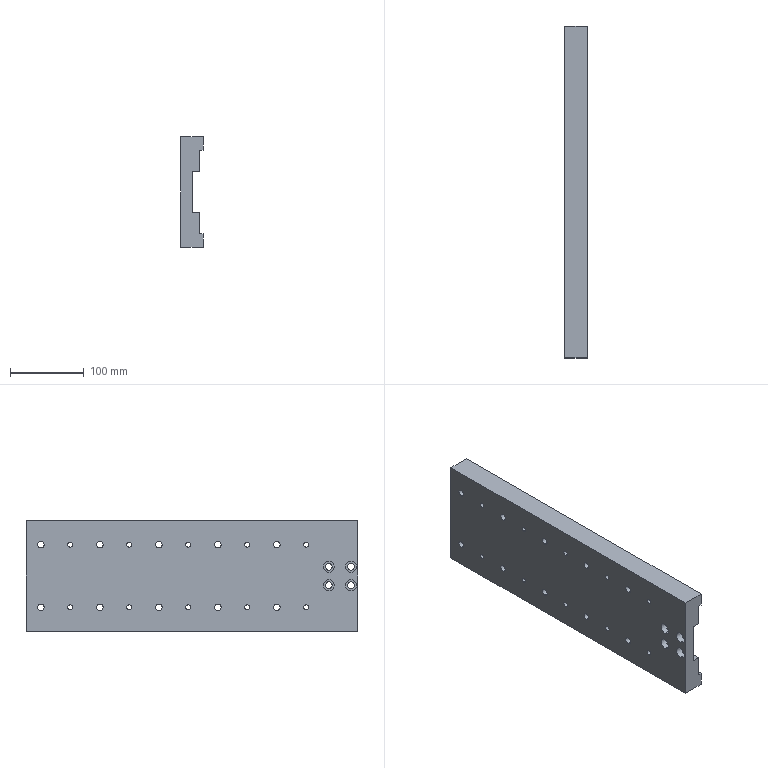Part | SolidWorks | features HoleWzd 3, ICE 2, LPattern 2, Extrusion 1 | 1 solid | 104 faces | box 30 x 450 x 150 mm | volume 1472324 mm3 | cylinder 76 | plane 28 | commonest cylinder face diameters 9 x28 15 x28 6.8 x20